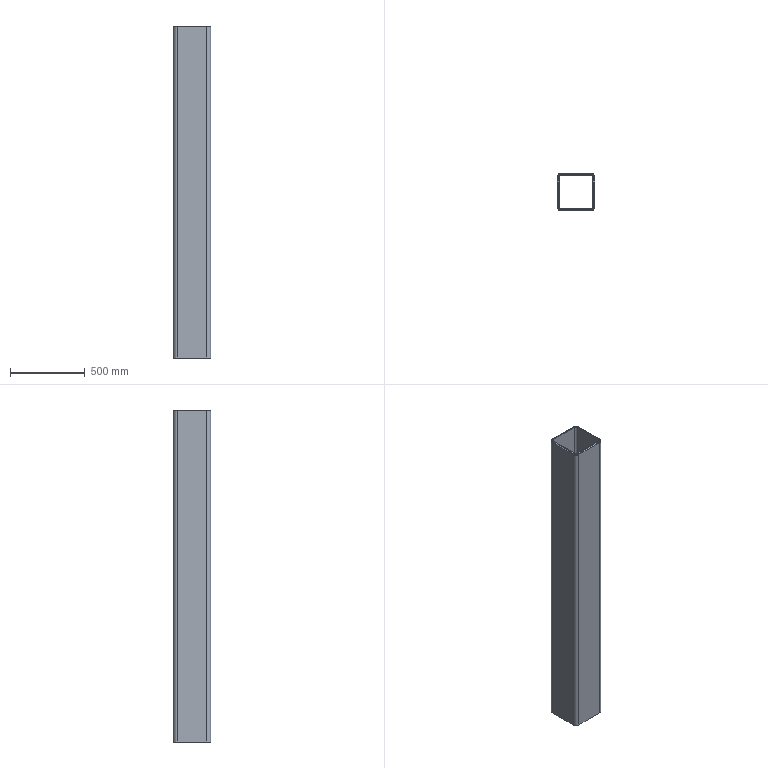Part | SolidWorks | features Chamfer 1, Extrusion 1, ICE 1, RefAxis 1 | 1 solid | 30 faces | box 250 x 250 x 2220 mm | volume 24230431 mm3 | plane 16 | cylinder 10 | cone 4 | commonest cylinder face diameters 28 x4 52 x4 80 x2
STEP:
#1=CARTESIAN_POINT('',(-120.,99.,2220.));
#2=VERTEX_POINT('',#1);
#3=CARTESIAN_POINT('',(-120.,-99.,2220.));
#4=VERTEX_POINT('',#3);
#5=CARTESIAN_POINT('',(-120.,99.,2220.));
#6=DIRECTION('',(0.,-1.,0.));
#7=VECTOR('',#6,1000.);
#8=LINE('',#5,#7);
#9=EDGE_CURVE('',#2,#4,#8,.T.);
#10=ORIENTED_EDGE('',*,*,#9,.T.);
#11=CARTESIAN_POINT('',(-99.,-120.,2220.));
#12=VERTEX_POINT('',#11);
#13=CARTESIAN_POINT('',(-99.,-99.,2220.));
#14=DIRECTION('',(0.,0.,1.));
#15=DIRECTION('',(-1.,0.,0.));
#16=AXIS2_PLACEMENT_3D('',#13,#14,#15);
#17=CIRCLE('',#16,21.);
#18=EDGE_CURVE('',#4,#12,#17,.T.);
#19=ORIENTED_EDGE('',*,*,#18,.T.);
#20=CARTESIAN_POINT('',(99.,-120.,2220.));
#21=VERTEX_POINT('',#20);
#22=CARTESIAN_POINT('',(-99.,-120.,2220.));
#23=DIRECTION('',(1.,0.,0.));
#24=VECTOR('',#23,1000.);
#25=LINE('',#22,#24);
#26=EDGE_CURVE('',#12,#21,#25,.T.);
#27=ORIENTED_EDGE('',*,*,#26,.T.);
#28=CARTESIAN_POINT('',(120.,-99.,2220.));
#29=VERTEX_POINT('',#28);
#30=CARTESIAN_POINT('',(99.,-99.,2220.));
#31=DIRECTION('',(0.,0.,1.));
#32=DIRECTION('',(-1.,0.,0.));
#33=AXIS2_PLACEMENT_3D('',#30,#31,#32);
#34=CIRCLE('',#33,21.);
#35=EDGE_CURVE('',#21,#29,#34,.T.);
#36=ORIENTED_EDGE('',*,*,#35,.T.);
#37=CARTESIAN_POINT('',(120.,99.,2220.));
#38=VERTEX_POINT('',#37);
#39=CARTESIAN_POINT('',(120.,99.,2220.));
#40=DIRECTION('',(0.,1.,0.));
#41=VECTOR('',#40,1000.);
#42=LINE('',#39,#41);
#43=EDGE_CURVE('',#29,#38,#42,.T.);
#44=ORIENTED_EDGE('',*,*,#43,.T.);
#45=CARTESIAN_POINT('',(99.,120.,2220.));
#46=VERTEX_POINT('',#45);
#47=CARTESIAN_POINT('',(99.,99.,2220.));
#48=DIRECTION('',(0.,0.,1.));
#49=DIRECTION('',(-1.,0.,0.));
#50=AXIS2_PLACEMENT_3D('',#47,#48,#49);
#51=CIRCLE('',#50,21.);
#52=EDGE_CURVE('',#38,#46,#51,.T.);
#53=ORIENTED_EDGE('',*,*,#52,.T.);
#54=CARTESIAN_POINT('',(-99.,120.,2220.));
#55=VERTEX_POINT('',#54);
#56=CARTESIAN_POINT('',(-99.,120.,2220.));
#57=DIRECTION('',(-1.,0.,0.));
#58=VECTOR('',#57,1000.);
#59=LINE('',#56,#58);
#60=EDGE_CURVE('',#46,#55,#59,.T.);
#61=ORIENTED_EDGE('',*,*,#60,.T.);
#62=CARTESIAN_POINT('',(-99.,99.,2220.));
#63=DIRECTION('',(0.,0.,1.));
#64=DIRECTION('',(-1.,0.,0.));
#65=AXIS2_PLACEMENT_3D('',#62,#63,#64);
#66=CIRCLE('',#65,21.);
#67=EDGE_CURVE('',#55,#2,#66,.T.);
#68=ORIENTED_EDGE('',*,*,#67,.T.);
#69=EDGE_LOOP('',(#10,#19,#27,#36,#44,#53,#61,#68));
#70=FACE_OUTER_BOUND('',#69,.T.);
#71=CARTESIAN_POINT('',(-113.,-99.,2220.));
#72=VERTEX_POINT('',#71);
#73=CARTESIAN_POINT('',(-99.,-113.,2220.));
#74=VERTEX_POINT('',#73);
#75=CARTESIAN_POINT('',(-99.,-99.,2220.));
#76=DIRECTION('',(0.,0.,1.));
#77=DIRECTION('',(-1.,0.,0.));
#78=AXIS2_PLACEMENT_3D('',#75,#76,#77);
#79=CIRCLE('',#78,14.);
#80=EDGE_CURVE('',#72,#74,#79,.T.);
#81=ORIENTED_EDGE('',*,*,#80,.F.);
#82=CARTESIAN_POINT('',(-113.,99.,2220.));
#83=VERTEX_POINT('',#82);
#84=CARTESIAN_POINT('',(-113.,99.,2220.));
#85=DIRECTION('',(0.,-1.,0.));
#86=VECTOR('',#85,1000.);
#87=LINE('',#84,#86);
#88=EDGE_CURVE('',#83,#72,#87,.T.);
#89=ORIENTED_EDGE('',*,*,#88,.F.);
#90=CARTESIAN_POINT('',(-99.,113.,2220.));
#91=VERTEX_POINT('',#90);
#92=CARTESIAN_POINT('',(-99.,99.,2220.));
#93=DIRECTION('',(0.,0.,1.));
#94=DIRECTION('',(-1.,0.,0.));
#95=AXIS2_PLACEMENT_3D('',#92,#93,#94);
#96=CIRCLE('',#95,14.);
#97=EDGE_CURVE('',#91,#83,#96,.T.);
#98=ORIENTED_EDGE('',*,*,#97,.F.);
#99=CARTESIAN_POINT('',(99.,113.,2220.));
#100=VERTEX_POINT('',#99);
#101=CARTESIAN_POINT('',(-99.,113.,2220.));
#102=DIRECTION('',(-1.,0.,0.));
#103=VECTOR('',#102,1000.);
#104=LINE('',#101,#103);
#105=EDGE_CURVE('',#100,#91,#104,.T.);
#106=ORIENTED_EDGE('',*,*,#105,.F.);
#107=CARTESIAN_POINT('',(113.,99.,2220.));
#108=VERTEX_POINT('',#107);
#109=CARTESIAN_POINT('',(99.,99.,2220.));
#110=DIRECTION('',(0.,0.,1.));
#111=DIRECTION('',(1.,0.,0.));
#112=AXIS2_PLACEMENT_3D('',#109,#110,#111);
#113=CIRCLE('',#112,14.);
#114=EDGE_CURVE('',#108,#100,#113,.T.);
#115=ORIENTED_EDGE('',*,*,#114,.F.);
#116=CARTESIAN_POINT('',(113.,-99.,2220.));
#117=VERTEX_POINT('',#116);
#118=CARTESIAN_POINT('',(113.,99.,2220.));
#119=DIRECTION('',(0.,1.,0.));
#120=VECTOR('',#119,1000.);
#121=LINE('',#118,#120);
#122=EDGE_CURVE('',#117,#108,#121,.T.);
#123=ORIENTED_EDGE('',*,*,#122,.F.);
#124=CARTESIAN_POINT('',(99.,-113.,2220.));
#125=VERTEX_POINT('',#124);
#126=CARTESIAN_POINT('',(99.,-99.,2220.));
#127=DIRECTION('',(0.,0.,1.));
#128=DIRECTION('',(1.,0.,0.));
#129=AXIS2_PLACEMENT_3D('',#126,#127,#128);
#130=CIRCLE('',#129,14.);
#131=EDGE_CURVE('',#125,#117,#130,.T.);
#132=ORIENTED_EDGE('',*,*,#131,.F.);
#133=CARTESIAN_POINT('',(-99.,-113.,2220.));
#134=DIRECTION('',(1.,0.,0.));
#135=VECTOR('',#134,1000.);
#136=LINE('',#133,#135);
#137=EDGE_CURVE('',#74,#125,#136,.T.);
#138=ORIENTED_EDGE('',*,*,#137,.F.);
#139=EDGE_LOOP('',(#81,#89,#98,#106,#115,#123,#132,#138));
#140=FACE_BOUND('',#139,.T.);
#141=CARTESIAN_POINT('',(-99.,99.,2220.));
#142=DIRECTION('',(0.,0.,-1.));
#143=DIRECTION('',(-1.,0.,0.));
#144=AXIS2_PLACEMENT_3D('',#141,#142,#143);
#145=PLANE('',#144);
#146=ADVANCED_FACE('',(#70,#140),#145,.F.);
#147=CARTESIAN_POINT('',(-99.,125.,0.));
#148=VERTEX_POINT('',#147);
#149=CARTESIAN_POINT('',(-125.,99.,0.));
#150=VERTEX_POINT('',#149);
#151=CARTESIAN_POINT('',(-99.,99.,0.));
#152=DIRECTION('',(0.,0.,1.));
#153=DIRECTION('',(-1.,0.,0.));
#154=AXIS2_PLACEMENT_3D('',#151,#152,#153);
#155=CIRCLE('',#154,26.);
#156=EDGE_CURVE('',#148,#150,#155,.T.);
#157=ORIENTED_EDGE('',*,*,#156,.F.);
#158=CARTESIAN_POINT('',(99.,125.,0.));
#159=VERTEX_POINT('',#158);
#160=CARTESIAN_POINT('',(-99.,125.,0.));
#161=DIRECTION('',(-1.,0.,0.));
#162=VECTOR('',#161,1000.);
#163=LINE('',#160,#162);
#164=EDGE_CURVE('',#159,#148,#163,.T.);
#165=ORIENTED_EDGE('',*,*,#164,.F.);
#166=CARTESIAN_POINT('',(125.,99.,0.));
#167=VERTEX_POINT('',#166);
#168=CARTESIAN_POINT('',(99.,99.,0.));
#169=DIRECTION('',(0.,0.,1.));
#170=DIRECTION('',(1.,0.,0.));
#171=AXIS2_PLACEMENT_3D('',#168,#169,#170);
#172=CIRCLE('',#171,26.);
#173=EDGE_CURVE('',#167,#159,#172,.T.);
#174=ORIENTED_EDGE('',*,*,#173,.F.);
#175=CARTESIAN_POINT('',(125.,-99.,0.));
#176=VERTEX_POINT('',#175);
#177=CARTESIAN_POINT('',(125.,99.,0.));
#178=DIRECTION('',(0.,1.,0.));
#179=VECTOR('',#178,1000.);
#180=LINE('',#177,#179);
#181=EDGE_CURVE('',#176,#167,#180,.T.);
#182=ORIENTED_EDGE('',*,*,#181,.F.);
#183=CARTESIAN_POINT('',(99.,-125.,0.));
#184=VERTEX_POINT('',#183);
#185=CARTESIAN_POINT('',(99.,-99.,0.));
#186=DIRECTION('',(0.,0.,1.));
#187=DIRECTION('',(1.,0.,0.));
#188=AXIS2_PLACEMENT_3D('',#185,#186,#187);
#189=CIRCLE('',#188,26.);
#190=EDGE_CURVE('',#184,#176,#189,.T.);
#191=ORIENTED_EDGE('',*,*,#190,.F.);
#192=CARTESIAN_POINT('',(-99.,-125.,0.));
#193=VERTEX_POINT('',#192);
#194=CARTESIAN_POINT('',(-99.,-125.,0.));
#195=DIRECTION('',(1.,0.,0.));
#196=VECTOR('',#195,1000.);
#197=LINE('',#194,#196);
#198=EDGE_CURVE('',#193,#184,#197,.T.);
#199=ORIENTED_EDGE('',*,*,#198,.F.);
#200=CARTESIAN_POINT('',(-125.,-99.,0.));
#201=VERTEX_POINT('',#200);
#202=CARTESIAN_POINT('',(-99.,-99.,0.));
#203=DIRECTION('',(0.,0.,1.));
#204=DIRECTION('',(-1.,0.,0.));
#205=AXIS2_PLACEMENT_3D('',#202,#203,#204);
#206=CIRCLE('',#205,26.);
#207=EDGE_CURVE('',#201,#193,#206,.T.);
#208=ORIENTED_EDGE('',*,*,#207,.F.);
#209=CARTESIAN_POINT('',(-125.,99.,0.));
#210=DIRECTION('',(0.,-1.,0.));
#211=VECTOR('',#210,1000.);
#212=LINE('',#209,#211);
#213=EDGE_CURVE('',#150,#201,#212,.T.);
#214=ORIENTED_EDGE('',*,*,#213,.F.);
#215=EDGE_LOOP('',(#157,#165,#174,#182,#191,#199,#208,#214));
#216=FACE_OUTER_BOUND('',#215,.T.);
#217=CARTESIAN_POINT('',(-113.,99.,0.));
#218=VERTEX_POINT('',#217);
#219=CARTESIAN_POINT('',(-113.,-99.,0.));
#220=VERTEX_POINT('',#219);
#221=CARTESIAN_POINT('',(-113.,99.,0.));
#222=DIRECTION('',(0.,-1.,0.));
#223=VECTOR('',#222,1000.);
#224=LINE('',#221,#223);
#225=EDGE_CURVE('',#218,#220,#224,.T.);
#226=ORIENTED_EDGE('',*,*,#225,.T.);
#227=CARTESIAN_POINT('',(-99.,-113.,0.));
#228=VERTEX_POINT('',#227);
#229=CARTESIAN_POINT('',(-99.,-99.,0.));
#230=DIRECTION('',(0.,0.,1.));
#231=DIRECTION('',(-1.,0.,0.));
#232=AXIS2_PLACEMENT_3D('',#229,#230,#231);
#233=CIRCLE('',#232,14.);
#234=EDGE_CURVE('',#220,#228,#233,.T.);
#235=ORIENTED_EDGE('',*,*,#234,.T.);
#236=CARTESIAN_POINT('',(99.,-113.,0.));
#237=VERTEX_POINT('',#236);
#238=CARTESIAN_POINT('',(-99.,-113.,0.));
#239=DIRECTION('',(1.,0.,0.));
#240=VECTOR('',#239,1000.);
#241=LINE('',#238,#240);
#242=EDGE_CURVE('',#228,#237,#241,.T.);
#243=ORIENTED_EDGE('',*,*,#242,.T.);
#244=CARTESIAN_POINT('',(113.,-99.,0.));
#245=VERTEX_POINT('',#244);
#246=CARTESIAN_POINT('',(99.,-99.,0.));
#247=DIRECTION('',(0.,0.,1.));
#248=DIRECTION('',(1.,0.,0.));
#249=AXIS2_PLACEMENT_3D('',#246,#247,#248);
#250=CIRCLE('',#249,14.);
#251=EDGE_CURVE('',#237,#245,#250,.T.);
#252=ORIENTED_EDGE('',*,*,#251,.T.);
#253=CARTESIAN_POINT('',(113.,99.,0.));
#254=VERTEX_POINT('',#253);
#255=CARTESIAN_POINT('',(113.,99.,0.));
#256=DIRECTION('',(0.,1.,0.));
#257=VECTOR('',#256,1000.);
#258=LINE('',#255,#257);
#259=EDGE_CURVE('',#245,#254,#258,.T.);
#260=ORIENTED_EDGE('',*,*,#259,.T.);
#261=CARTESIAN_POINT('',(99.,113.,0.));
#262=VERTEX_POINT('',#261);
#263=CARTESIAN_POINT('',(99.,99.,0.));
#264=DIRECTION('',(0.,0.,1.));
#265=DIRECTION('',(1.,0.,0.));
#266=AXIS2_PLACEMENT_3D('',#263,#264,#265);
#267=CIRCLE('',#266,14.);
#268=EDGE_CURVE('',#254,#262,#267,.T.);
#269=ORIENTED_EDGE('',*,*,#268,.T.);
#270=CARTESIAN_POINT('',(-99.,113.,0.));
#271=VERTEX_POINT('',#270);
#272=CARTESIAN_POINT('',(-99.,113.,0.));
#273=DIRECTION('',(-1.,0.,0.));
#274=VECTOR('',#273,1000.);
#275=LINE('',#272,#274);
#276=EDGE_CURVE('',#262,#271,#275,.T.);
#277=ORIENTED_EDGE('',*,*,#276,.T.);
#278=CARTESIAN_POINT('',(-99.,99.,0.));
#279=DIRECTION('',(0.,0.,1.));
#280=DIRECTION('',(-1.,0.,0.));
#281=AXIS2_PLACEMENT_3D('',#278,#279,#280);
#282=CIRCLE('',#281,14.);
#283=EDGE_CURVE('',#271,#218,#282,.T.);
#284=ORIENTED_EDGE('',*,*,#283,.T.);
#285=EDGE_LOOP('',(#226,#235,#243,#252,#260,#269,#277,#284));
#286=FACE_BOUND('',#285,.T.);
#287=CARTESIAN_POINT('',(-99.,99.,0.));
#288=DIRECTION('',(0.,0.,-1.));
#289=DIRECTION('',(-1.,0.,0.));
#290=AXIS2_PLACEMENT_3D('',#287,#288,#289);
#291=PLANE('',#290);
#292=ADVANCED_FACE('',(#216,#286),#291,.T.);
#293=CARTESIAN_POINT('',(-125.,99.,2215.));
#294=VERTEX_POINT('',#293);
#295=CARTESIAN_POINT('',(-125.,99.,2220.));
#296=DIRECTION('',(0.,0.,-1.));
#297=VECTOR('',#296,1000.);
#298=LINE('',#295,#297);
#299=EDGE_CURVE('',#294,#150,#298,.T.);
#300=ORIENTED_EDGE('',*,*,#299,.F.);
#301=CARTESIAN_POINT('',(-99.,125.,2215.));
#302=VERTEX_POINT('',#301);
#303=CARTESIAN_POINT('',(-99.,99.,2215.));
#304=DIRECTION('',(0.,0.,-1.));
#305=DIRECTION('',(-1.,0.,0.));
#306=AXIS2_PLACEMENT_3D('',#303,#304,#305);
#307=CIRCLE('',#306,26.);
#308=EDGE_CURVE('',#294,#302,#307,.T.);
#309=ORIENTED_EDGE('',*,*,#308,.T.);
#310=CARTESIAN_POINT('',(-99.,125.,2220.));
#311=DIRECTION('',(0.,0.,-1.));
#312=VECTOR('',#311,1000.);
#313=LINE('',#310,#312);
#314=EDGE_CURVE('',#302,#148,#313,.T.);
#315=ORIENTED_EDGE('',*,*,#314,.T.);
#316=ORIENTED_EDGE('',*,*,#156,.T.);
#317=EDGE_LOOP('',(#300,#309,#315,#316));
#318=FACE_OUTER_BOUND('',#317,.T.);
#319=CARTESIAN_POINT('',(-99.,99.,2220.));
#320=DIRECTION('',(0.,0.,-1.));
#321=DIRECTION('',(-1.,0.,0.));
#322=AXIS2_PLACEMENT_3D('',#319,#320,#321);
#323=CYLINDRICAL_SURFACE('',#322,26.);
#324=ADVANCED_FACE('',(#318),#323,.T.);
#325=CARTESIAN_POINT('',(-125.,-99.,2215.));
#326=VERTEX_POINT('',#325);
#327=CARTESIAN_POINT('',(-125.,-99.,2220.));
#328=DIRECTION('',(0.,0.,-1.));
#329=VECTOR('',#328,1000.);
#330=LINE('',#327,#329);
#331=EDGE_CURVE('',#326,#201,#330,.T.);
#332=ORIENTED_EDGE('',*,*,#331,.F.);
#333=CARTESIAN_POINT('',(-125.,99.,2215.));
#334=DIRECTION('',(0.,1.,0.));
#335=VECTOR('',#334,1000.);
#336=LINE('',#333,#335);
#337=EDGE_CURVE('',#326,#294,#336,.T.);
#338=ORIENTED_EDGE('',*,*,#337,.T.);
#339=ORIENTED_EDGE('',*,*,#299,.T.);
#340=ORIENTED_EDGE('',*,*,#213,.T.);
#341=EDGE_LOOP('',(#332,#338,#339,#340));
#342=FACE_OUTER_BOUND('',#341,.T.);
#343=CARTESIAN_POINT('',(-125.,99.,2220.));
#344=DIRECTION('',(1.,0.,0.));
#345=DIRECTION('',(0.,1.,0.));
#346=AXIS2_PLACEMENT_3D('',#343,#344,#345);
#347=PLANE('',#346);
#348=ADVANCED_FACE('',(#342),#347,.F.);
#349=CARTESIAN_POINT('',(-99.,-125.,2215.));
#350=VERTEX_POINT('',#349);
#351=CARTESIAN_POINT('',(-99.,-125.,2220.));
#352=DIRECTION('',(0.,0.,-1.));
#353=VECTOR('',#352,1000.);
#354=LINE('',#351,#353);
#355=EDGE_CURVE('',#350,#193,#354,.T.);
#356=ORIENTED_EDGE('',*,*,#355,.F.);
#357=CARTESIAN_POINT('',(-99.,-99.,2215.));
#358=DIRECTION('',(0.,0.,-1.));
#359=DIRECTION('',(-1.,0.,0.));
#360=AXIS2_PLACEMENT_3D('',#357,#358,#359);
#361=CIRCLE('',#360,26.);
#362=EDGE_CURVE('',#350,#326,#361,.T.);
#363=ORIENTED_EDGE('',*,*,#362,.T.);
#364=ORIENTED_EDGE('',*,*,#331,.T.);
#365=ORIENTED_EDGE('',*,*,#207,.T.);
#366=EDGE_LOOP('',(#356,#363,#364,#365));
#367=FACE_OUTER_BOUND('',#366,.T.);
#368=CARTESIAN_POINT('',(-99.,-99.,2220.));
#369=DIRECTION('',(0.,0.,-1.));
#370=DIRECTION('',(-1.,0.,0.));
#371=AXIS2_PLACEMENT_3D('',#368,#369,#370);
#372=CYLINDRICAL_SURFACE('',#371,26.);
#373=ADVANCED_FACE('',(#367),#372,.T.);
#374=CARTESIAN_POINT('',(99.,-125.,2215.));
#375=VERTEX_POINT('',#374);
#376=CARTESIAN_POINT('',(99.,-125.,2220.));
#377=DIRECTION('',(0.,0.,-1.));
#378=VECTOR('',#377,1000.);
#379=LINE('',#376,#378);
#380=EDGE_CURVE('',#375,#184,#379,.T.);
#381=ORIENTED_EDGE('',*,*,#380,.F.);
#382=CARTESIAN_POINT('',(-99.,-125.,2215.));
#383=DIRECTION('',(-1.,0.,0.));
#384=VECTOR('',#383,1000.);
#385=LINE('',#382,#384);
#386=EDGE_CURVE('',#375,#350,#385,.T.);
#387=ORIENTED_EDGE('',*,*,#386,.T.);
#388=ORIENTED_EDGE('',*,*,#355,.T.);
#389=ORIENTED_EDGE('',*,*,#198,.T.);
#390=EDGE_LOOP('',(#381,#387,#388,#389));
#391=FACE_OUTER_BOUND('',#390,.T.);
#392=CARTESIAN_POINT('',(-99.,-125.,2220.));
#393=DIRECTION('',(0.,1.,0.));
#394=DIRECTION('',(0.,0.,1.));
#395=AXIS2_PLACEMENT_3D('',#392,#393,#394);
#396=PLANE('',#395);
#397=ADVANCED_FACE('',(#391),#396,.F.);
#398=CARTESIAN_POINT('',(125.,-99.,2215.));
#399=VERTEX_POINT('',#398);
#400=CARTESIAN_POINT('',(125.,-99.,2220.));
#401=DIRECTION('',(0.,0.,-1.));
#402=VECTOR('',#401,1000.);
#403=LINE('',#400,#402);
#404=EDGE_CURVE('',#399,#176,#403,.T.);
#405=ORIENTED_EDGE('',*,*,#404,.F.);
#406=CARTESIAN_POINT('',(99.,-99.,2215.));
#407=DIRECTION('',(0.,0.,-1.));
#408=DIRECTION('',(-1.,0.,0.));
#409=AXIS2_PLACEMENT_3D('',#406,#407,#408);
#410=CIRCLE('',#409,26.);
#411=EDGE_CURVE('',#399,#375,#410,.T.);
#412=ORIENTED_EDGE('',*,*,#411,.T.);
#413=ORIENTED_EDGE('',*,*,#380,.T.);
#414=ORIENTED_EDGE('',*,*,#190,.T.);
#415=EDGE_LOOP('',(#405,#412,#413,#414));
#416=FACE_OUTER_BOUND('',#415,.T.);
#417=CARTESIAN_POINT('',(99.,-99.,2220.));
#418=DIRECTION('',(0.,0.,-1.));
#419=DIRECTION('',(-1.,0.,0.));
#420=AXIS2_PLACEMENT_3D('',#417,#418,#419);
#421=CYLINDRICAL_SURFACE('',#420,26.);
#422=ADVANCED_FACE('',(#416),#421,.T.);
#423=CARTESIAN_POINT('',(125.,-40.,395.));
#424=VERTEX_POINT('',#423);
#425=CARTESIAN_POINT('',(125.,-40.,245.));
#426=VERTEX_POINT('',#425);
#427=CARTESIAN_POINT('',(125.,-40.,395.));
#428=DIRECTION('',(0.,0.,-1.));
#429=VECTOR('',#428,1000.);
#430=LINE('',#427,#429);
#431=EDGE_CURVE('',#424,#426,#430,.T.);
#432=ORIENTED_EDGE('',*,*,#431,.F.);
#433=CARTESIAN_POINT('',(125.,40.,395.));
#434=VERTEX_POINT('',#433);
#435=CARTESIAN_POINT('',(125.,0.,395.));
#436=DIRECTION('',(1.,0.,0.));
#437=DIRECTION('',(0.,1.,0.));
#438=AXIS2_PLACEMENT_3D('',#435,#436,#437);
#439=CIRCLE('',#438,40.);
#440=EDGE_CURVE('',#434,#424,#439,.T.);
#441=ORIENTED_EDGE('',*,*,#440,.F.);
#442=CARTESIAN_POINT('',(125.,40.,245.));
#443=VERTEX_POINT('',#442);
#444=CARTESIAN_POINT('',(125.,40.,395.));
#445=DIRECTION('',(0.,0.,1.));
#446=VECTOR('',#445,1000.);
#447=LINE('',#444,#446);
#448=EDGE_CURVE('',#443,#434,#447,.T.);
#449=ORIENTED_EDGE('',*,*,#448,.F.);
#450=CARTESIAN_POINT('',(125.,0.,245.));
#451=DIRECTION('',(1.,0.,0.));
#452=DIRECTION('',(0.,1.,0.));
#453=AXIS2_PLACEMENT_3D('',#450,#451,#452);
#454=CIRCLE('',#453,40.);
#455=EDGE_CURVE('',#426,#443,#454,.T.);
#456=ORIENTED_EDGE('',*,*,#455,.F.);
#457=EDGE_LOOP('',(#432,#441,#449,#456));
#458=FACE_BOUND('',#457,.T.);
#459=CARTESIAN_POINT('',(125.,99.,2215.));
#460=VERTEX_POINT('',#459);
#461=CARTESIAN_POINT('',(125.,99.,2220.));
#462=DIRECTION('',(0.,0.,-1.));
#463=VECTOR('',#462,1000.);
#464=LINE('',#461,#463);
#465=EDGE_CURVE('',#460,#167,#464,.T.);
#466=ORIENTED_EDGE('',*,*,#465,.F.);
#467=CARTESIAN_POINT('',(125.,99.,2215.));
#468=DIRECTION('',(0.,-1.,0.));
#469=VECTOR('',#468,1000.);
#470=LINE('',#467,#469);
#471=EDGE_CURVE('',#460,#399,#470,.T.);
#472=ORIENTED_EDGE('',*,*,#471,.T.);
#473=ORIENTED_EDGE('',*,*,#404,.T.);
#474=ORIENTED_EDGE('',*,*,#181,.T.);
#475=EDGE_LOOP('',(#466,#472,#473,#474));
#476=FACE_OUTER_BOUND('',#475,.T.);
#477=CARTESIAN_POINT('',(125.,99.,2220.));
#478=DIRECTION('',(-1.,0.,0.));
#479=DIRECTION('',(0.,-1.,0.));
#480=AXIS2_PLACEMENT_3D('',#477,#478,#479);
#481=PLANE('',#480);
#482=ADVANCED_FACE('',(#458,#476),#481,.F.);
#483=CARTESIAN_POINT('',(99.,125.,2215.));
#484=VERTEX_POINT('',#483);
#485=CARTESIAN_POINT('',(99.,125.,2220.));
#486=DIRECTION('',(0.,0.,-1.));
#487=VECTOR('',#486,1000.);
#488=LINE('',#485,#487);
#489=EDGE_CURVE('',#484,#159,#488,.T.);
#490=ORIENTED_EDGE('',*,*,#489,.F.);
#491=CARTESIAN_POINT('',(99.,99.,2215.));
#492=DIRECTION('',(0.,0.,-1.));
#493=DIRECTION('',(-1.,0.,0.));
#494=AXIS2_PLACEMENT_3D('',#491,#492,#493);
#495=CIRCLE('',#494,26.);
#496=EDGE_CURVE('',#484,#460,#495,.T.);
#497=ORIENTED_EDGE('',*,*,#496,.T.);
#498=ORIENTED_EDGE('',*,*,#465,.T.);
#499=ORIENTED_EDGE('',*,*,#173,.T.);
#500=EDGE_LOOP('',(#490,#497,#498,#499));
#501=FACE_OUTER_BOUND('',#500,.T.);
#502=CARTESIAN_POINT('',(99.,99.,2220.));
#503=DIRECTION('',(0.,0.,-1.));
#504=DIRECTION('',(-1.,0.,0.));
#505=AXIS2_PLACEMENT_3D('',#502,#503,#504);
#506=CYLINDRICAL_SURFACE('',#505,26.);
#507=ADVANCED_FACE('',(#501),#506,.T.);
#508=ORIENTED_EDGE('',*,*,#314,.F.);
#509=CARTESIAN_POINT('',(-99.,125.,2215.));
#510=DIRECTION('',(1.,0.,0.));
#511=VECTOR('',#510,1000.);
#512=LINE('',#509,#511);
#513=EDGE_CURVE('',#302,#484,#512,.T.);
#514=ORIENTED_EDGE('',*,*,#513,.T.);
#515=ORIENTED_EDGE('',*,*,#489,.T.);
#516=ORIENTED_EDGE('',*,*,#164,.T.);
#517=EDGE_LOOP('',(#508,#514,#515,#516));
#518=FACE_OUTER_BOUND('',#517,.T.);
#519=CARTESIAN_POINT('',(-99.,125.,2220.));
#520=DIRECTION('',(0.,-1.,0.));
#521=DIRECTION('',(0.,0.,-1.));
#522=AXIS2_PLACEMENT_3D('',#519,#520,#521);
#523=PLANE('',#522);
#524=ADVANCED_FACE('',(#518),#523,.F.);
#525=ORIENTED_EDGE('',*,*,#234,.F.);
#526=CARTESIAN_POINT('',(-113.,-99.,2220.));
#527=DIRECTION('',(0.,0.,-1.));
#528=VECTOR('',#527,1000.);
#529=LINE('',#526,#528);
#530=EDGE_CURVE('',#72,#220,#529,.T.);
#531=ORIENTED_EDGE('',*,*,#530,.F.);
#532=ORIENTED_EDGE('',*,*,#80,.T.);
#533=CARTESIAN_POINT('',(-99.,-113.,2220.));
#534=DIRECTION('',(0.,0.,-1.));
#535=VECTOR('',#534,1000.);
#536=LINE('',#533,#535);
#537=EDGE_CURVE('',#74,#228,#536,.T.);
#538=ORIENTED_EDGE('',*,*,#537,.T.);
#539=EDGE_LOOP('',(#525,#531,#532,#538));
#540=FACE_OUTER_BOUND('',#539,.T.);
#541=CARTESIAN_POINT('',(-99.,-99.,2220.));
#542=DIRECTION('',(0.,0.,-1.));
#543=DIRECTION('',(-1.,0.,0.));
#544=AXIS2_PLACEMENT_3D('',#541,#542,#543);
#545=CYLINDRICAL_SURFACE('',#544,14.);
#546=ADVANCED_FACE('',(#540),#545,.F.);
#547=ORIENTED_EDGE('',*,*,#242,.F.);
#548=ORIENTED_EDGE('',*,*,#537,.F.);
#549=ORIENTED_EDGE('',*,*,#137,.T.);
#550=CARTESIAN_POINT('',(99.,-113.,2220.));
#551=DIRECTION('',(0.,0.,-1.));
#552=VECTOR('',#551,1000.);
#553=LINE('',#550,#552);
#554=EDGE_CURVE('',#125,#237,#553,.T.);
#555=ORIENTED_EDGE('',*,*,#554,.T.);
#556=EDGE_LOOP('',(#547,#548,#549,#555));
#557=FACE_OUTER_BOUND('',#556,.T.);
#558=CARTESIAN_POINT('',(-99.,-113.,2220.));
#559=DIRECTION('',(0.,1.,0.));
#560=DIRECTION('',(0.,0.,1.));
#561=AXIS2_PLACEMENT_3D('',#558,#559,#560);
#562=PLANE('',#561);
#563=ADVANCED_FACE('',(#557),#562,.T.);
#564=ORIENTED_EDGE('',*,*,#251,.F.);
#565=ORIENTED_EDGE('',*,*,#554,.F.);
#566=ORIENTED_EDGE('',*,*,#131,.T.);
#567=CARTESIAN_POINT('',(113.,-99.,2220.));
#568=DIRECTION('',(0.,0.,-1.));
#569=VECTOR('',#568,1000.);
#570=LINE('',#567,#569);
#571=EDGE_CURVE('',#117,#245,#570,.T.);
#572=ORIENTED_EDGE('',*,*,#571,.T.);
#573=EDGE_LOOP('',(#564,#565,#566,#572));
#574=FACE_OUTER_BOUND('',#573,.T.);
#575=CARTESIAN_POINT('',(99.,-99.,2220.));
#576=DIRECTION('',(0.,0.,-1.));
#577=DIRECTION('',(-1.,0.,0.));
#578=AXIS2_PLACEMENT_3D('',#575,#576,#577);
#579=CYLINDRICAL_SURFACE('',#578,14.);
#580=ADVANCED_FACE('',(#574),#579,.F.);
#581=CARTESIAN_POINT('',(113.,40.,395.));
#582=VERTEX_POINT('',#581);
#583=CARTESIAN_POINT('',(113.,-40.,395.));
#584=VERTEX_POINT('',#583);
#585=CARTESIAN_POINT('',(113.,0.,395.));
#586=DIRECTION('',(1.,0.,0.));
#587=DIRECTION('',(0.,-1.,0.));
#588=AXIS2_PLACEMENT_3D('',#585,#586,#587);
#589=CIRCLE('',#588,40.);
#590=EDGE_CURVE('',#582,#584,#589,.T.);
#591=ORIENTED_EDGE('',*,*,#590,.T.);
#592=CARTESIAN_POINT('',(113.,-40.,245.));
#593=VERTEX_POINT('',#592);
#594=CARTESIAN_POINT('',(113.,-40.,395.));
#595=DIRECTION('',(0.,0.,-1.));
#596=VECTOR('',#595,1000.);
#597=LINE('',#594,#596);
#598=EDGE_CURVE('',#584,#593,#597,.T.);
#599=ORIENTED_EDGE('',*,*,#598,.T.);
#600=CARTESIAN_POINT('',(113.,40.,245.));
#601=VERTEX_POINT('',#600);
#602=CARTESIAN_POINT('',(113.,0.,245.));
#603=DIRECTION('',(1.,0.,0.));
#604=DIRECTION('',(0.,-1.,0.));
#605=AXIS2_PLACEMENT_3D('',#602,#603,#604);
#606=CIRCLE('',#605,40.);
#607=EDGE_CURVE('',#593,#601,#606,.T.);
#608=ORIENTED_EDGE('',*,*,#607,.T.);
#609=CARTESIAN_POINT('',(113.,40.,395.));
#610=DIRECTION('',(0.,0.,1.));
#611=VECTOR('',#610,1000.);
#612=LINE('',#609,#611);
#613=EDGE_CURVE('',#601,#582,#612,.T.);
#614=ORIENTED_EDGE('',*,*,#613,.T.);
#615=EDGE_LOOP('',(#591,#599,#608,#614));
#616=FACE_BOUND('',#615,.T.);
#617=ORIENTED_EDGE('',*,*,#259,.F.);
#618=ORIENTED_EDGE('',*,*,#571,.F.);
#619=ORIENTED_EDGE('',*,*,#122,.T.);
#620=CARTESIAN_POINT('',(113.,99.,2220.));
#621=DIRECTION('',(0.,0.,-1.));
#622=VECTOR('',#621,1000.);
#623=LINE('',#620,#622);
#624=EDGE_CURVE('',#108,#254,#623,.T.);
#625=ORIENTED_EDGE('',*,*,#624,.T.);
#626=EDGE_LOOP('',(#617,#618,#619,#625));
#627=FACE_OUTER_BOUND('',#626,.T.);
#628=CARTESIAN_POINT('',(113.,99.,2220.));
#629=DIRECTION('',(-1.,0.,0.));
#630=DIRECTION('',(0.,-1.,0.));
#631=AXIS2_PLACEMENT_3D('',#628,#629,#630);
#632=PLANE('',#631);
#633=ADVANCED_FACE('',(#616,#627),#632,.T.);
#634=ORIENTED_EDGE('',*,*,#268,.F.);
#635=ORIENTED_EDGE('',*,*,#624,.F.);
#636=ORIENTED_EDGE('',*,*,#114,.T.);
#637=CARTESIAN_POINT('',(99.,113.,2220.));
#638=DIRECTION('',(0.,0.,-1.));
#639=VECTOR('',#638,1000.);
#640=LINE('',#637,#639);
#641=EDGE_CURVE('',#100,#262,#640,.T.);
#642=ORIENTED_EDGE('',*,*,#641,.T.);
#643=EDGE_LOOP('',(#634,#635,#636,#642));
#644=FACE_OUTER_BOUND('',#643,.T.);
#645=CARTESIAN_POINT('',(99.,99.,2220.));
#646=DIRECTION('',(0.,0.,-1.));
#647=DIRECTION('',(-1.,0.,0.));
#648=AXIS2_PLACEMENT_3D('',#645,#646,#647);
#649=CYLINDRICAL_SURFACE('',#648,14.);
#650=ADVANCED_FACE('',(#644),#649,.F.);
#651=ORIENTED_EDGE('',*,*,#276,.F.);
#652=ORIENTED_EDGE('',*,*,#641,.F.);
#653=ORIENTED_EDGE('',*,*,#105,.T.);
#654=CARTESIAN_POINT('',(-99.,113.,2220.));
#655=DIRECTION('',(0.,0.,-1.));
#656=VECTOR('',#655,1000.);
#657=LINE('',#654,#656);
#658=EDGE_CURVE('',#91,#271,#657,.T.);
#659=ORIENTED_EDGE('',*,*,#658,.T.);
#660=EDGE_LOOP('',(#651,#652,#653,#659));
#661=FACE_OUTER_BOUND('',#660,.T.);
#662=CARTESIAN_POINT('',(-99.,113.,2220.));
#663=DIRECTION('',(0.,-1.,0.));
#664=DIRECTION('',(0.,0.,-1.));
#665=AXIS2_PLACEMENT_3D('',#662,#663,#664);
#666=PLANE('',#665);
#667=ADVANCED_FACE('',(#661),#666,.T.);
#668=ORIENTED_EDGE('',*,*,#283,.F.);
#669=ORIENTED_EDGE('',*,*,#658,.F.);
#670=ORIENTED_EDGE('',*,*,#97,.T.);
#671=CARTESIAN_POINT('',(-113.,99.,2220.));
#672=DIRECTION('',(0.,0.,-1.));
#673=VECTOR('',#672,1000.);
#674=LINE('',#671,#673);
#675=EDGE_CURVE('',#83,#218,#674,.T.);
#676=ORIENTED_EDGE('',*,*,#675,.T.);
#677=EDGE_LOOP('',(#668,#669,#670,#676));
#678=FACE_OUTER_BOUND('',#677,.T.);
#679=CARTESIAN_POINT('',(-99.,99.,2220.));
#680=DIRECTION('',(0.,0.,-1.));
#681=DIRECTION('',(-1.,0.,0.));
#682=AXIS2_PLACEMENT_3D('',#679,#680,#681);
#683=CYLINDRICAL_SURFACE('',#682,14.);
#684=ADVANCED_FACE('',(#678),#683,.F.);
#685=ORIENTED_EDGE('',*,*,#225,.F.);
#686=ORIENTED_EDGE('',*,*,#675,.F.);
#687=ORIENTED_EDGE('',*,*,#88,.T.);
#688=ORIENTED_EDGE('',*,*,#530,.T.);
#689=EDGE_LOOP('',(#685,#686,#687,#688));
#690=FACE_OUTER_BOUND('',#689,.T.);
#691=CARTESIAN_POINT('',(-113.,99.,2220.));
#692=DIRECTION('',(1.,0.,0.));
#693=DIRECTION('',(0.,1.,0.));
#694=AXIS2_PLACEMENT_3D('',#691,#692,#693);
#695=PLANE('',#694);
#696=ADVANCED_FACE('',(#690),#695,.T.);
#697=CARTESIAN_POINT('',(125.,99.,2215.));
#698=DIRECTION('',(-0.7071,0.,0.7071));
#699=VECTOR('',#698,1000.);
#700=LINE('',#697,#699);
#701=EDGE_CURVE('',#460,#38,#700,.T.);
#702=ORIENTED_EDGE('',*,*,#701,.F.);
#703=ORIENTED_EDGE('',*,*,#496,.F.);
#704=CARTESIAN_POINT('',(99.,120.,2220.));
#705=DIRECTION('',(0.,0.7071,-0.7071));
#706=VECTOR('',#705,1000.);
#707=LINE('',#704,#706);
#708=EDGE_CURVE('',#46,#484,#707,.T.);
#709=ORIENTED_EDGE('',*,*,#708,.F.);
#710=ORIENTED_EDGE('',*,*,#52,.F.);
#711=EDGE_LOOP('',(#702,#703,#709,#710));
#712=FACE_OUTER_BOUND('',#711,.T.);
#713=CARTESIAN_POINT('',(99.,99.,2220.));
#714=DIRECTION('',(0.,0.,-1.));
#715=DIRECTION('',(-1.,0.,0.));
#716=AXIS2_PLACEMENT_3D('',#713,#714,#715);
#717=CONICAL_SURFACE('',#716,21.,0.7854);
#718=ADVANCED_FACE('',(#712),#717,.T.);
#719=ORIENTED_EDGE('',*,*,#708,.T.);
#720=ORIENTED_EDGE('',*,*,#513,.F.);
#721=CARTESIAN_POINT('',(-99.,120.,2220.));
#722=DIRECTION('',(0.,0.7071,-0.7071));
#723=VECTOR('',#722,1000.);
#724=LINE('',#721,#723);
#725=EDGE_CURVE('',#55,#302,#724,.T.);
#726=ORIENTED_EDGE('',*,*,#725,.F.);
#727=ORIENTED_EDGE('',*,*,#60,.F.);
#728=EDGE_LOOP('',(#719,#720,#726,#727));
#729=FACE_OUTER_BOUND('',#728,.T.);
#730=CARTESIAN_POINT('',(-99.,120.,2220.));
#731=DIRECTION('',(0.,-0.7071,-0.7071));
#732=DIRECTION('',(-1.,0.,0.));
#733=AXIS2_PLACEMENT_3D('',#730,#731,#732);
#734=PLANE('',#733);
#735=ADVANCED_FACE('',(#729),#734,.F.);
#736=ORIENTED_EDGE('',*,*,#701,.T.);
#737=ORIENTED_EDGE('',*,*,#43,.F.);
#738=CARTESIAN_POINT('',(125.,-99.,2215.));
#739=DIRECTION('',(-0.7071,0.,0.7071));
#740=VECTOR('',#739,1000.);
#741=LINE('',#738,#740);
#742=EDGE_CURVE('',#399,#29,#741,.T.);
#743=ORIENTED_EDGE('',*,*,#742,.F.);
#744=ORIENTED_EDGE('',*,*,#471,.F.);
#745=EDGE_LOOP('',(#736,#737,#743,#744));
#746=FACE_OUTER_BOUND('',#745,.T.);
#747=CARTESIAN_POINT('',(120.,99.,2220.));
#748=DIRECTION('',(-0.7071,0.,-0.7071));
#749=DIRECTION('',(0.,1.,0.));
#750=AXIS2_PLACEMENT_3D('',#747,#748,#749);
#751=PLANE('',#750);
#752=ADVANCED_FACE('',(#746),#751,.F.);
#753=ORIENTED_EDGE('',*,*,#725,.T.);
#754=ORIENTED_EDGE('',*,*,#308,.F.);
#755=CARTESIAN_POINT('',(-120.,99.,2220.));
#756=DIRECTION('',(-0.7071,0.,-0.7071));
#757=VECTOR('',#756,1000.);
#758=LINE('',#755,#757);
#759=EDGE_CURVE('',#2,#294,#758,.T.);
#760=ORIENTED_EDGE('',*,*,#759,.F.);
#761=ORIENTED_EDGE('',*,*,#67,.F.);
#762=EDGE_LOOP('',(#753,#754,#760,#761));
#763=FACE_OUTER_BOUND('',#762,.T.);
#764=CARTESIAN_POINT('',(-99.,99.,2220.));
#765=DIRECTION('',(0.,0.,-1.));
#766=DIRECTION('',(-1.,0.,0.));
#767=AXIS2_PLACEMENT_3D('',#764,#765,#766);
#768=CONICAL_SURFACE('',#767,21.,0.7854);
#769=ADVANCED_FACE('',(#763),#768,.T.);
#770=ORIENTED_EDGE('',*,*,#742,.T.);
#771=ORIENTED_EDGE('',*,*,#35,.F.);
#772=CARTESIAN_POINT('',(99.,-125.,2215.));
#773=DIRECTION('',(0.,0.7071,0.7071));
#774=VECTOR('',#773,1000.);
#775=LINE('',#772,#774);
#776=EDGE_CURVE('',#375,#21,#775,.T.);
#777=ORIENTED_EDGE('',*,*,#776,.F.);
#778=ORIENTED_EDGE('',*,*,#411,.F.);
#779=EDGE_LOOP('',(#770,#771,#777,#778));
#780=FACE_OUTER_BOUND('',#779,.T.);
#781=CARTESIAN_POINT('',(99.,-99.,2220.));
#782=DIRECTION('',(0.,0.,-1.));
#783=DIRECTION('',(-1.,0.,0.));
#784=AXIS2_PLACEMENT_3D('',#781,#782,#783);
#785=CONICAL_SURFACE('',#784,21.,0.7854);
#786=ADVANCED_FACE('',(#780),#785,.T.);
#787=ORIENTED_EDGE('',*,*,#759,.T.);
#788=ORIENTED_EDGE('',*,*,#337,.F.);
#789=CARTESIAN_POINT('',(-120.,-99.,2220.));
#790=DIRECTION('',(-0.7071,0.,-0.7071));
#791=VECTOR('',#790,1000.);
#792=LINE('',#789,#791);
#793=EDGE_CURVE('',#4,#326,#792,.T.);
#794=ORIENTED_EDGE('',*,*,#793,.F.);
#795=ORIENTED_EDGE('',*,*,#9,.F.);
#796=EDGE_LOOP('',(#787,#788,#794,#795));
#797=FACE_OUTER_BOUND('',#796,.T.);
#798=CARTESIAN_POINT('',(-120.,99.,2220.));
#799=DIRECTION('',(0.7071,0.,-0.7071));
#800=DIRECTION('',(0.,-1.,0.));
#801=AXIS2_PLACEMENT_3D('',#798,#799,#800);
#802=PLANE('',#801);
#803=ADVANCED_FACE('',(#797),#802,.F.);
#804=ORIENTED_EDGE('',*,*,#776,.T.);
#805=ORIENTED_EDGE('',*,*,#26,.F.);
#806=CARTESIAN_POINT('',(-99.,-125.,2215.));
#807=DIRECTION('',(0.,0.7071,0.7071));
#808=VECTOR('',#807,1000.);
#809=LINE('',#806,#808);
#810=EDGE_CURVE('',#350,#12,#809,.T.);
#811=ORIENTED_EDGE('',*,*,#810,.F.);
#812=ORIENTED_EDGE('',*,*,#386,.F.);
#813=EDGE_LOOP('',(#804,#805,#811,#812));
#814=FACE_OUTER_BOUND('',#813,.T.);
#815=CARTESIAN_POINT('',(-99.,-120.,2220.));
#816=DIRECTION('',(0.,0.7071,-0.7071));
#817=DIRECTION('',(1.,0.,0.));
#818=AXIS2_PLACEMENT_3D('',#815,#816,#817);
#819=PLANE('',#818);
#820=ADVANCED_FACE('',(#814),#819,.F.);
#821=ORIENTED_EDGE('',*,*,#793,.T.);
#822=ORIENTED_EDGE('',*,*,#362,.F.);
#823=ORIENTED_EDGE('',*,*,#810,.T.);
#824=ORIENTED_EDGE('',*,*,#18,.F.);
#825=EDGE_LOOP('',(#821,#822,#823,#824));
#826=FACE_OUTER_BOUND('',#825,.T.);
#827=CARTESIAN_POINT('',(-99.,-99.,2220.));
#828=DIRECTION('',(0.,0.,-1.));
#829=DIRECTION('',(-1.,0.,0.));
#830=AXIS2_PLACEMENT_3D('',#827,#828,#829);
#831=CONICAL_SURFACE('',#830,21.,0.7854);
#832=ADVANCED_FACE('',(#826),#831,.T.);
#833=CARTESIAN_POINT('',(-125.001,40.,395.));
#834=DIRECTION('',(1.,0.,0.));
#835=VECTOR('',#834,1000.);
#836=LINE('',#833,#835);
#837=EDGE_CURVE('',#582,#434,#836,.T.);
#838=ORIENTED_EDGE('',*,*,#837,.T.);
#839=ORIENTED_EDGE('',*,*,#440,.T.);
#840=CARTESIAN_POINT('',(-125.001,-40.,395.));
#841=DIRECTION('',(1.,0.,0.));
#842=VECTOR('',#841,1000.);
#843=LINE('',#840,#842);
#844=EDGE_CURVE('',#584,#424,#843,.T.);
#845=ORIENTED_EDGE('',*,*,#844,.F.);
#846=ORIENTED_EDGE('',*,*,#590,.F.);
#847=EDGE_LOOP('',(#838,#839,#845,#846));
#848=FACE_OUTER_BOUND('',#847,.T.);
#849=CARTESIAN_POINT('',(-125.001,0.,395.));
#850=DIRECTION('',(1.,0.,0.));
#851=DIRECTION('',(0.,1.,0.));
#852=AXIS2_PLACEMENT_3D('',#849,#850,#851);
#853=CYLINDRICAL_SURFACE('',#852,40.);
#854=ADVANCED_FACE('',(#848),#853,.F.);
#855=CARTESIAN_POINT('',(-125.001,40.,245.));
#856=DIRECTION('',(1.,0.,0.));
#857=VECTOR('',#856,1000.);
#858=LINE('',#855,#857);
#859=EDGE_CURVE('',#601,#443,#858,.T.);
#860=ORIENTED_EDGE('',*,*,#859,.T.);
#861=ORIENTED_EDGE('',*,*,#448,.T.);
#862=ORIENTED_EDGE('',*,*,#837,.F.);
#863=ORIENTED_EDGE('',*,*,#613,.F.);
#864=EDGE_LOOP('',(#860,#861,#862,#863));
#865=FACE_OUTER_BOUND('',#864,.T.);
#866=CARTESIAN_POINT('',(-125.001,40.,395.));
#867=DIRECTION('',(0.,1.,0.));
#868=DIRECTION('',(-1.,0.,0.));
#869=AXIS2_PLACEMENT_3D('',#866,#867,#868);
#870=PLANE('',#869);
#871=ADVANCED_FACE('',(#865),#870,.F.);
#872=CARTESIAN_POINT('',(-125.001,-40.,245.));
#873=DIRECTION('',(1.,0.,0.));
#874=VECTOR('',#873,1000.);
#875=LINE('',#872,#874);
#876=EDGE_CURVE('',#593,#426,#875,.T.);
#877=ORIENTED_EDGE('',*,*,#876,.T.);
#878=ORIENTED_EDGE('',*,*,#455,.T.);
#879=ORIENTED_EDGE('',*,*,#859,.F.);
#880=ORIENTED_EDGE('',*,*,#607,.F.);
#881=EDGE_LOOP('',(#877,#878,#879,#880));
#882=FACE_OUTER_BOUND('',#881,.T.);
#883=CARTESIAN_POINT('',(-125.001,0.,245.));
#884=DIRECTION('',(1.,0.,0.));
#885=DIRECTION('',(0.,1.,0.));
#886=AXIS2_PLACEMENT_3D('',#883,#884,#885);
#887=CYLINDRICAL_SURFACE('',#886,40.);
#888=ADVANCED_FACE('',(#882),#887,.F.);
#889=ORIENTED_EDGE('',*,*,#844,.T.);
#890=ORIENTED_EDGE('',*,*,#431,.T.);
#891=ORIENTED_EDGE('',*,*,#876,.F.);
#892=ORIENTED_EDGE('',*,*,#598,.F.);
#893=EDGE_LOOP('',(#889,#890,#891,#892));
#894=FACE_OUTER_BOUND('',#893,.T.);
#895=CARTESIAN_POINT('',(-125.001,-40.,395.));
#896=DIRECTION('',(0.,-1.,0.));
#897=DIRECTION('',(1.,0.,0.));
#898=AXIS2_PLACEMENT_3D('',#895,#896,#897);
#899=PLANE('',#898);
#900=ADVANCED_FACE('',(#894),#899,.F.);
#901=CLOSED_SHELL('',(#146,#292,#324,#348,#373,#397,#422,#482,#507,#524,#546,#563,#580,#633,#650,#667,#684,#696,#718,#735,#752,#769,#786,#803,#820,#832,#854,#871,#888,#900));
#902=MANIFOLD_SOLID_BREP('',#901);
#903=CARTESIAN_POINT('',(0.,0.,0.));
#904=DIRECTION('',(0.,0.,1.));
#905=DIRECTION('',(1.,0.,0.));
#906=AXIS2_PLACEMENT_3D('',#903,#904,#905);
#907=(LENGTH_UNIT()NAMED_UNIT(*)SI_UNIT(.MILLI.,.METRE.));
#908=UNCERTAINTY_MEASURE_WITH_UNIT(LENGTH_MEASURE(0.00001),#907,'','');
#909=(NAMED_UNIT(*)PLANE_ANGLE_UNIT()SI_UNIT($,.RADIAN.));
#910=(NAMED_UNIT(*)SI_UNIT($,.STERADIAN.)SOLID_ANGLE_UNIT());
#911=(GEOMETRIC_REPRESENTATION_CONTEXT(3)GLOBAL_UNCERTAINTY_ASSIGNED_CONTEXT((#908))GLOBAL_UNIT_ASSIGNED_CONTEXT((#907,#909,#910))REPRESENTATION_CONTEXT('',''));
#912=ADVANCED_BREP_SHAPE_REPRESENTATION('',(#902,#906),#911);